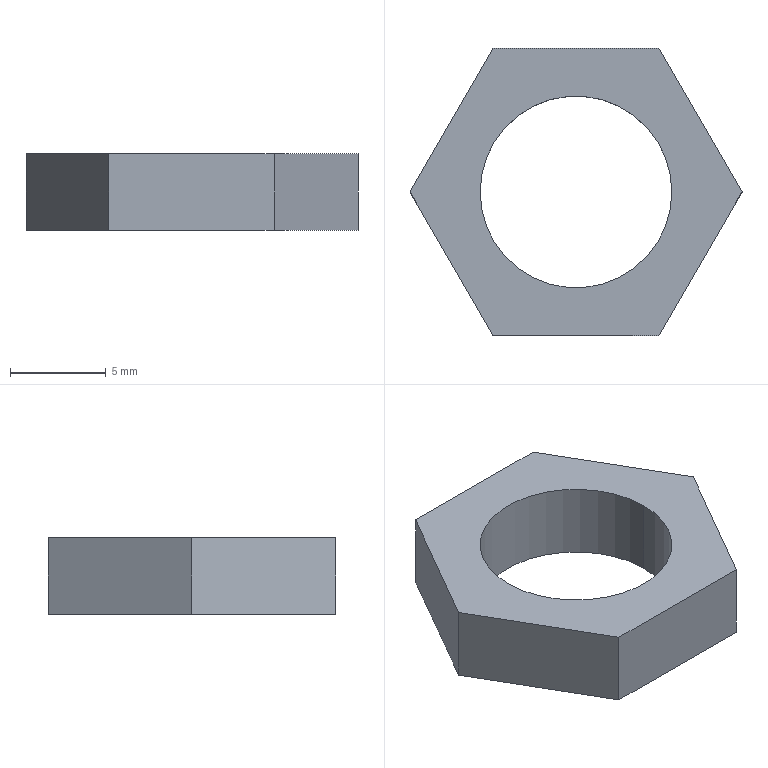Part | SolidWorks | features BaseBody 1 | 1 solid | 10 faces | box 17.321 x 15 x 4 mm | volume 465.264 mm3 | plane 8 | cylinder 2 | commonest cylinder face diameters 10 x2
STEP:
#1=CARTESIAN_POINT('',(5.,0.,4.));
#2=VERTEX_POINT('',#1);
#3=CARTESIAN_POINT('',(-5.,0.,4.));
#4=VERTEX_POINT('',#3);
#5=CARTESIAN_POINT('',(0.,0.,4.));
#6=DIRECTION('',(0.,0.,-1.));
#7=DIRECTION('',(-1.,0.,0.));
#8=AXIS2_PLACEMENT_3D('',#5,#6,#7);
#9=CIRCLE('',#8,5.);
#10=EDGE_CURVE('',#2,#4,#9,.T.);
#11=ORIENTED_EDGE('',*,*,#10,.F.);
#12=CARTESIAN_POINT('',(5.,0.,0.));
#13=VERTEX_POINT('',#12);
#14=CARTESIAN_POINT('',(5.,0.,0.));
#15=DIRECTION('',(0.,0.,-1.));
#16=VECTOR('',#15,1000.);
#17=LINE('',#14,#16);
#18=EDGE_CURVE('',#2,#13,#17,.T.);
#19=ORIENTED_EDGE('',*,*,#18,.T.);
#20=CARTESIAN_POINT('',(-5.,0.,0.));
#21=VERTEX_POINT('',#20);
#22=CARTESIAN_POINT('',(0.,0.,0.));
#23=DIRECTION('',(0.,0.,1.));
#24=DIRECTION('',(-1.,0.,0.));
#25=AXIS2_PLACEMENT_3D('',#22,#23,#24);
#26=CIRCLE('',#25,5.);
#27=EDGE_CURVE('',#21,#13,#26,.T.);
#28=ORIENTED_EDGE('',*,*,#27,.F.);
#29=CARTESIAN_POINT('',(-5.,0.,0.));
#30=DIRECTION('',(0.,0.,-1.));
#31=VECTOR('',#30,1000.);
#32=LINE('',#29,#31);
#33=EDGE_CURVE('',#4,#21,#32,.T.);
#34=ORIENTED_EDGE('',*,*,#33,.F.);
#35=EDGE_LOOP('',(#11,#19,#28,#34));
#36=FACE_OUTER_BOUND('',#35,.T.);
#37=CARTESIAN_POINT('',(0.,0.,0.));
#38=DIRECTION('',(0.,0.,-1.));
#39=DIRECTION('',(-1.,0.,0.));
#40=AXIS2_PLACEMENT_3D('',#37,#38,#39);
#41=CYLINDRICAL_SURFACE('',#40,5.);
#42=ADVANCED_FACE('',(#36),#41,.F.);
#43=CARTESIAN_POINT('',(-4.33,-7.5,0.));
#44=VERTEX_POINT('',#43);
#45=CARTESIAN_POINT('',(-8.66,0.,0.));
#46=VERTEX_POINT('',#45);
#47=CARTESIAN_POINT('',(-4.33,-7.5,0.));
#48=DIRECTION('',(-0.5,0.866,0.));
#49=VECTOR('',#48,1000.);
#50=LINE('',#47,#49);
#51=EDGE_CURVE('',#44,#46,#50,.T.);
#52=ORIENTED_EDGE('',*,*,#51,.F.);
#53=CARTESIAN_POINT('',(-4.33,-7.5,4.));
#54=VERTEX_POINT('',#53);
#55=CARTESIAN_POINT('',(-4.33,-7.5,0.));
#56=DIRECTION('',(0.,0.,1.));
#57=VECTOR('',#56,1000.);
#58=LINE('',#55,#57);
#59=EDGE_CURVE('',#44,#54,#58,.T.);
#60=ORIENTED_EDGE('',*,*,#59,.T.);
#61=CARTESIAN_POINT('',(-8.66,0.,4.));
#62=VERTEX_POINT('',#61);
#63=CARTESIAN_POINT('',(-4.33,-7.5,4.));
#64=DIRECTION('',(0.5,-0.866,0.));
#65=VECTOR('',#64,1000.);
#66=LINE('',#63,#65);
#67=EDGE_CURVE('',#62,#54,#66,.T.);
#68=ORIENTED_EDGE('',*,*,#67,.F.);
#69=CARTESIAN_POINT('',(-8.66,0.,0.));
#70=DIRECTION('',(0.,0.,1.));
#71=VECTOR('',#70,1000.);
#72=LINE('',#69,#71);
#73=EDGE_CURVE('',#46,#62,#72,.T.);
#74=ORIENTED_EDGE('',*,*,#73,.F.);
#75=EDGE_LOOP('',(#52,#60,#68,#74));
#76=FACE_OUTER_BOUND('',#75,.T.);
#77=CARTESIAN_POINT('',(-8.66,0.,0.));
#78=DIRECTION('',(-0.866,-0.5,0.));
#79=DIRECTION('',(-0.5,0.866,0.));
#80=AXIS2_PLACEMENT_3D('',#77,#78,#79);
#81=PLANE('',#80);
#82=ADVANCED_FACE('',(#76),#81,.T.);
#83=CARTESIAN_POINT('',(-4.33,7.5,0.));
#84=VERTEX_POINT('',#83);
#85=CARTESIAN_POINT('',(-8.66,0.,0.));
#86=DIRECTION('',(0.5,0.866,0.));
#87=VECTOR('',#86,1000.);
#88=LINE('',#85,#87);
#89=EDGE_CURVE('',#46,#84,#88,.T.);
#90=ORIENTED_EDGE('',*,*,#89,.F.);
#91=ORIENTED_EDGE('',*,*,#73,.T.);
#92=CARTESIAN_POINT('',(-4.33,7.5,4.));
#93=VERTEX_POINT('',#92);
#94=CARTESIAN_POINT('',(-8.66,0.,4.));
#95=DIRECTION('',(-0.5,-0.866,0.));
#96=VECTOR('',#95,1000.);
#97=LINE('',#94,#96);
#98=EDGE_CURVE('',#93,#62,#97,.T.);
#99=ORIENTED_EDGE('',*,*,#98,.F.);
#100=CARTESIAN_POINT('',(-4.33,7.5,0.));
#101=DIRECTION('',(0.,0.,1.));
#102=VECTOR('',#101,1000.);
#103=LINE('',#100,#102);
#104=EDGE_CURVE('',#84,#93,#103,.T.);
#105=ORIENTED_EDGE('',*,*,#104,.F.);
#106=EDGE_LOOP('',(#90,#91,#99,#105));
#107=FACE_OUTER_BOUND('',#106,.T.);
#108=CARTESIAN_POINT('',(-4.33,7.5,0.));
#109=DIRECTION('',(-0.866,0.5,0.));
#110=DIRECTION('',(0.,0.,1.));
#111=AXIS2_PLACEMENT_3D('',#108,#109,#110);
#112=PLANE('',#111);
#113=ADVANCED_FACE('',(#107),#112,.T.);
#114=CARTESIAN_POINT('',(4.33,7.5,0.));
#115=VERTEX_POINT('',#114);
#116=CARTESIAN_POINT('',(-4.33,7.5,0.));
#117=DIRECTION('',(1.,0.,0.));
#118=VECTOR('',#117,1000.);
#119=LINE('',#116,#118);
#120=EDGE_CURVE('',#84,#115,#119,.T.);
#121=ORIENTED_EDGE('',*,*,#120,.F.);
#122=ORIENTED_EDGE('',*,*,#104,.T.);
#123=CARTESIAN_POINT('',(4.33,7.5,4.));
#124=VERTEX_POINT('',#123);
#125=CARTESIAN_POINT('',(-4.33,7.5,4.));
#126=DIRECTION('',(-1.,0.,0.));
#127=VECTOR('',#126,1000.);
#128=LINE('',#125,#127);
#129=EDGE_CURVE('',#124,#93,#128,.T.);
#130=ORIENTED_EDGE('',*,*,#129,.F.);
#131=CARTESIAN_POINT('',(4.33,7.5,0.));
#132=DIRECTION('',(0.,0.,1.));
#133=VECTOR('',#132,1000.);
#134=LINE('',#131,#133);
#135=EDGE_CURVE('',#115,#124,#134,.T.);
#136=ORIENTED_EDGE('',*,*,#135,.F.);
#137=EDGE_LOOP('',(#121,#122,#130,#136));
#138=FACE_OUTER_BOUND('',#137,.T.);
#139=CARTESIAN_POINT('',(4.33,7.5,0.));
#140=DIRECTION('',(0.,1.,0.));
#141=DIRECTION('',(1.,0.,0.));
#142=AXIS2_PLACEMENT_3D('',#139,#140,#141);
#143=PLANE('',#142);
#144=ADVANCED_FACE('',(#138),#143,.T.);
#145=CARTESIAN_POINT('',(8.66,0.,0.));
#146=VERTEX_POINT('',#145);
#147=CARTESIAN_POINT('',(4.33,7.5,0.));
#148=DIRECTION('',(0.5,-0.866,0.));
#149=VECTOR('',#148,1000.);
#150=LINE('',#147,#149);
#151=EDGE_CURVE('',#115,#146,#150,.T.);
#152=ORIENTED_EDGE('',*,*,#151,.F.);
#153=ORIENTED_EDGE('',*,*,#135,.T.);
#154=CARTESIAN_POINT('',(8.66,0.,4.));
#155=VERTEX_POINT('',#154);
#156=CARTESIAN_POINT('',(4.33,7.5,4.));
#157=DIRECTION('',(-0.5,0.866,0.));
#158=VECTOR('',#157,1000.);
#159=LINE('',#156,#158);
#160=EDGE_CURVE('',#155,#124,#159,.T.);
#161=ORIENTED_EDGE('',*,*,#160,.F.);
#162=CARTESIAN_POINT('',(8.66,0.,0.));
#163=DIRECTION('',(0.,0.,1.));
#164=VECTOR('',#163,1000.);
#165=LINE('',#162,#164);
#166=EDGE_CURVE('',#146,#155,#165,.T.);
#167=ORIENTED_EDGE('',*,*,#166,.F.);
#168=EDGE_LOOP('',(#152,#153,#161,#167));
#169=FACE_OUTER_BOUND('',#168,.T.);
#170=CARTESIAN_POINT('',(8.66,0.,0.));
#171=DIRECTION('',(0.866,0.5,0.));
#172=DIRECTION('',(0.,0.,-1.));
#173=AXIS2_PLACEMENT_3D('',#170,#171,#172);
#174=PLANE('',#173);
#175=ADVANCED_FACE('',(#169),#174,.T.);
#176=CARTESIAN_POINT('',(4.33,-7.5,0.));
#177=VERTEX_POINT('',#176);
#178=CARTESIAN_POINT('',(8.66,0.,0.));
#179=DIRECTION('',(-0.5,-0.866,0.));
#180=VECTOR('',#179,1000.);
#181=LINE('',#178,#180);
#182=EDGE_CURVE('',#146,#177,#181,.T.);
#183=ORIENTED_EDGE('',*,*,#182,.F.);
#184=ORIENTED_EDGE('',*,*,#166,.T.);
#185=CARTESIAN_POINT('',(4.33,-7.5,4.));
#186=VERTEX_POINT('',#185);
#187=CARTESIAN_POINT('',(8.66,0.,4.));
#188=DIRECTION('',(0.5,0.866,0.));
#189=VECTOR('',#188,1000.);
#190=LINE('',#187,#189);
#191=EDGE_CURVE('',#186,#155,#190,.T.);
#192=ORIENTED_EDGE('',*,*,#191,.F.);
#193=CARTESIAN_POINT('',(4.33,-7.5,0.));
#194=DIRECTION('',(0.,0.,1.));
#195=VECTOR('',#194,1000.);
#196=LINE('',#193,#195);
#197=EDGE_CURVE('',#177,#186,#196,.T.);
#198=ORIENTED_EDGE('',*,*,#197,.F.);
#199=EDGE_LOOP('',(#183,#184,#192,#198));
#200=FACE_OUTER_BOUND('',#199,.T.);
#201=CARTESIAN_POINT('',(4.33,-7.5,0.));
#202=DIRECTION('',(0.866,-0.5,0.));
#203=DIRECTION('',(0.,0.,-1.));
#204=AXIS2_PLACEMENT_3D('',#201,#202,#203);
#205=PLANE('',#204);
#206=ADVANCED_FACE('',(#200),#205,.T.);
#207=CARTESIAN_POINT('',(4.33,-7.5,0.));
#208=DIRECTION('',(-1.,0.,0.));
#209=VECTOR('',#208,1000.);
#210=LINE('',#207,#209);
#211=EDGE_CURVE('',#177,#44,#210,.T.);
#212=ORIENTED_EDGE('',*,*,#211,.F.);
#213=ORIENTED_EDGE('',*,*,#197,.T.);
#214=CARTESIAN_POINT('',(4.33,-7.5,4.));
#215=DIRECTION('',(1.,0.,0.));
#216=VECTOR('',#215,1000.);
#217=LINE('',#214,#216);
#218=EDGE_CURVE('',#54,#186,#217,.T.);
#219=ORIENTED_EDGE('',*,*,#218,.F.);
#220=ORIENTED_EDGE('',*,*,#59,.F.);
#221=EDGE_LOOP('',(#212,#213,#219,#220));
#222=FACE_OUTER_BOUND('',#221,.T.);
#223=CARTESIAN_POINT('',(-4.33,-7.5,0.));
#224=DIRECTION('',(0.,-1.,0.));
#225=DIRECTION('',(-1.,0.,0.));
#226=AXIS2_PLACEMENT_3D('',#223,#224,#225);
#227=PLANE('',#226);
#228=ADVANCED_FACE('',(#222),#227,.T.);
#229=ORIENTED_EDGE('',*,*,#27,.T.);
#230=CARTESIAN_POINT('',(0.,0.,0.));
#231=DIRECTION('',(0.,0.,1.));
#232=DIRECTION('',(-1.,0.,0.));
#233=AXIS2_PLACEMENT_3D('',#230,#231,#232);
#234=CIRCLE('',#233,5.);
#235=EDGE_CURVE('',#13,#21,#234,.T.);
#236=ORIENTED_EDGE('',*,*,#235,.T.);
#237=EDGE_LOOP('',(#229,#236));
#238=FACE_BOUND('',#237,.T.);
#239=ORIENTED_EDGE('',*,*,#211,.T.);
#240=ORIENTED_EDGE('',*,*,#51,.T.);
#241=ORIENTED_EDGE('',*,*,#89,.T.);
#242=ORIENTED_EDGE('',*,*,#120,.T.);
#243=ORIENTED_EDGE('',*,*,#151,.T.);
#244=ORIENTED_EDGE('',*,*,#182,.T.);
#245=EDGE_LOOP('',(#239,#240,#241,#242,#243,#244));
#246=FACE_OUTER_BOUND('',#245,.T.);
#247=CARTESIAN_POINT('',(0.,0.,0.));
#248=DIRECTION('',(0.,0.,1.));
#249=DIRECTION('',(1.,0.,0.));
#250=AXIS2_PLACEMENT_3D('',#247,#248,#249);
#251=PLANE('',#250);
#252=ADVANCED_FACE('',(#238,#246),#251,.F.);
#253=CARTESIAN_POINT('',(0.,0.,4.));
#254=DIRECTION('',(0.,0.,-1.));
#255=DIRECTION('',(-1.,0.,0.));
#256=AXIS2_PLACEMENT_3D('',#253,#254,#255);
#257=CIRCLE('',#256,5.);
#258=EDGE_CURVE('',#4,#2,#257,.T.);
#259=ORIENTED_EDGE('',*,*,#258,.T.);
#260=ORIENTED_EDGE('',*,*,#10,.T.);
#261=EDGE_LOOP('',(#259,#260));
#262=FACE_BOUND('',#261,.T.);
#263=ORIENTED_EDGE('',*,*,#218,.T.);
#264=ORIENTED_EDGE('',*,*,#191,.T.);
#265=ORIENTED_EDGE('',*,*,#160,.T.);
#266=ORIENTED_EDGE('',*,*,#129,.T.);
#267=ORIENTED_EDGE('',*,*,#98,.T.);
#268=ORIENTED_EDGE('',*,*,#67,.T.);
#269=EDGE_LOOP('',(#263,#264,#265,#266,#267,#268));
#270=FACE_OUTER_BOUND('',#269,.T.);
#271=CARTESIAN_POINT('',(0.,0.,4.));
#272=DIRECTION('',(0.,0.,1.));
#273=DIRECTION('',(1.,0.,0.));
#274=AXIS2_PLACEMENT_3D('',#271,#272,#273);
#275=PLANE('',#274);
#276=ADVANCED_FACE('',(#262,#270),#275,.T.);
#277=ORIENTED_EDGE('',*,*,#18,.F.);
#278=ORIENTED_EDGE('',*,*,#258,.F.);
#279=ORIENTED_EDGE('',*,*,#33,.T.);
#280=ORIENTED_EDGE('',*,*,#235,.F.);
#281=EDGE_LOOP('',(#277,#278,#279,#280));
#282=FACE_OUTER_BOUND('',#281,.T.);
#283=CARTESIAN_POINT('',(0.,0.,0.));
#284=DIRECTION('',(0.,0.,-1.));
#285=DIRECTION('',(-1.,0.,0.));
#286=AXIS2_PLACEMENT_3D('',#283,#284,#285);
#287=CYLINDRICAL_SURFACE('',#286,5.);
#288=ADVANCED_FACE('',(#282),#287,.F.);
#289=CLOSED_SHELL('',(#42,#82,#113,#144,#175,#206,#228,#252,#276,#288));
#290=MANIFOLD_SOLID_BREP('',#289);
#291=CARTESIAN_POINT('',(0.,0.,0.));
#292=DIRECTION('',(0.,0.,1.));
#293=DIRECTION('',(1.,0.,0.));
#294=AXIS2_PLACEMENT_3D('',#291,#292,#293);
#295=(LENGTH_UNIT()NAMED_UNIT(*)SI_UNIT(.MILLI.,.METRE.));
#296=UNCERTAINTY_MEASURE_WITH_UNIT(LENGTH_MEASURE(0.00001),#295,'','');
#297=(NAMED_UNIT(*)PLANE_ANGLE_UNIT()SI_UNIT($,.RADIAN.));
#298=(NAMED_UNIT(*)SI_UNIT($,.STERADIAN.)SOLID_ANGLE_UNIT());
#299=(GEOMETRIC_REPRESENTATION_CONTEXT(3)GLOBAL_UNCERTAINTY_ASSIGNED_CONTEXT((#296))GLOBAL_UNIT_ASSIGNED_CONTEXT((#295,#297,#298))REPRESENTATION_CONTEXT('',''));
#300=ADVANCED_BREP_SHAPE_REPRESENTATION('',(#290,#294),#299);